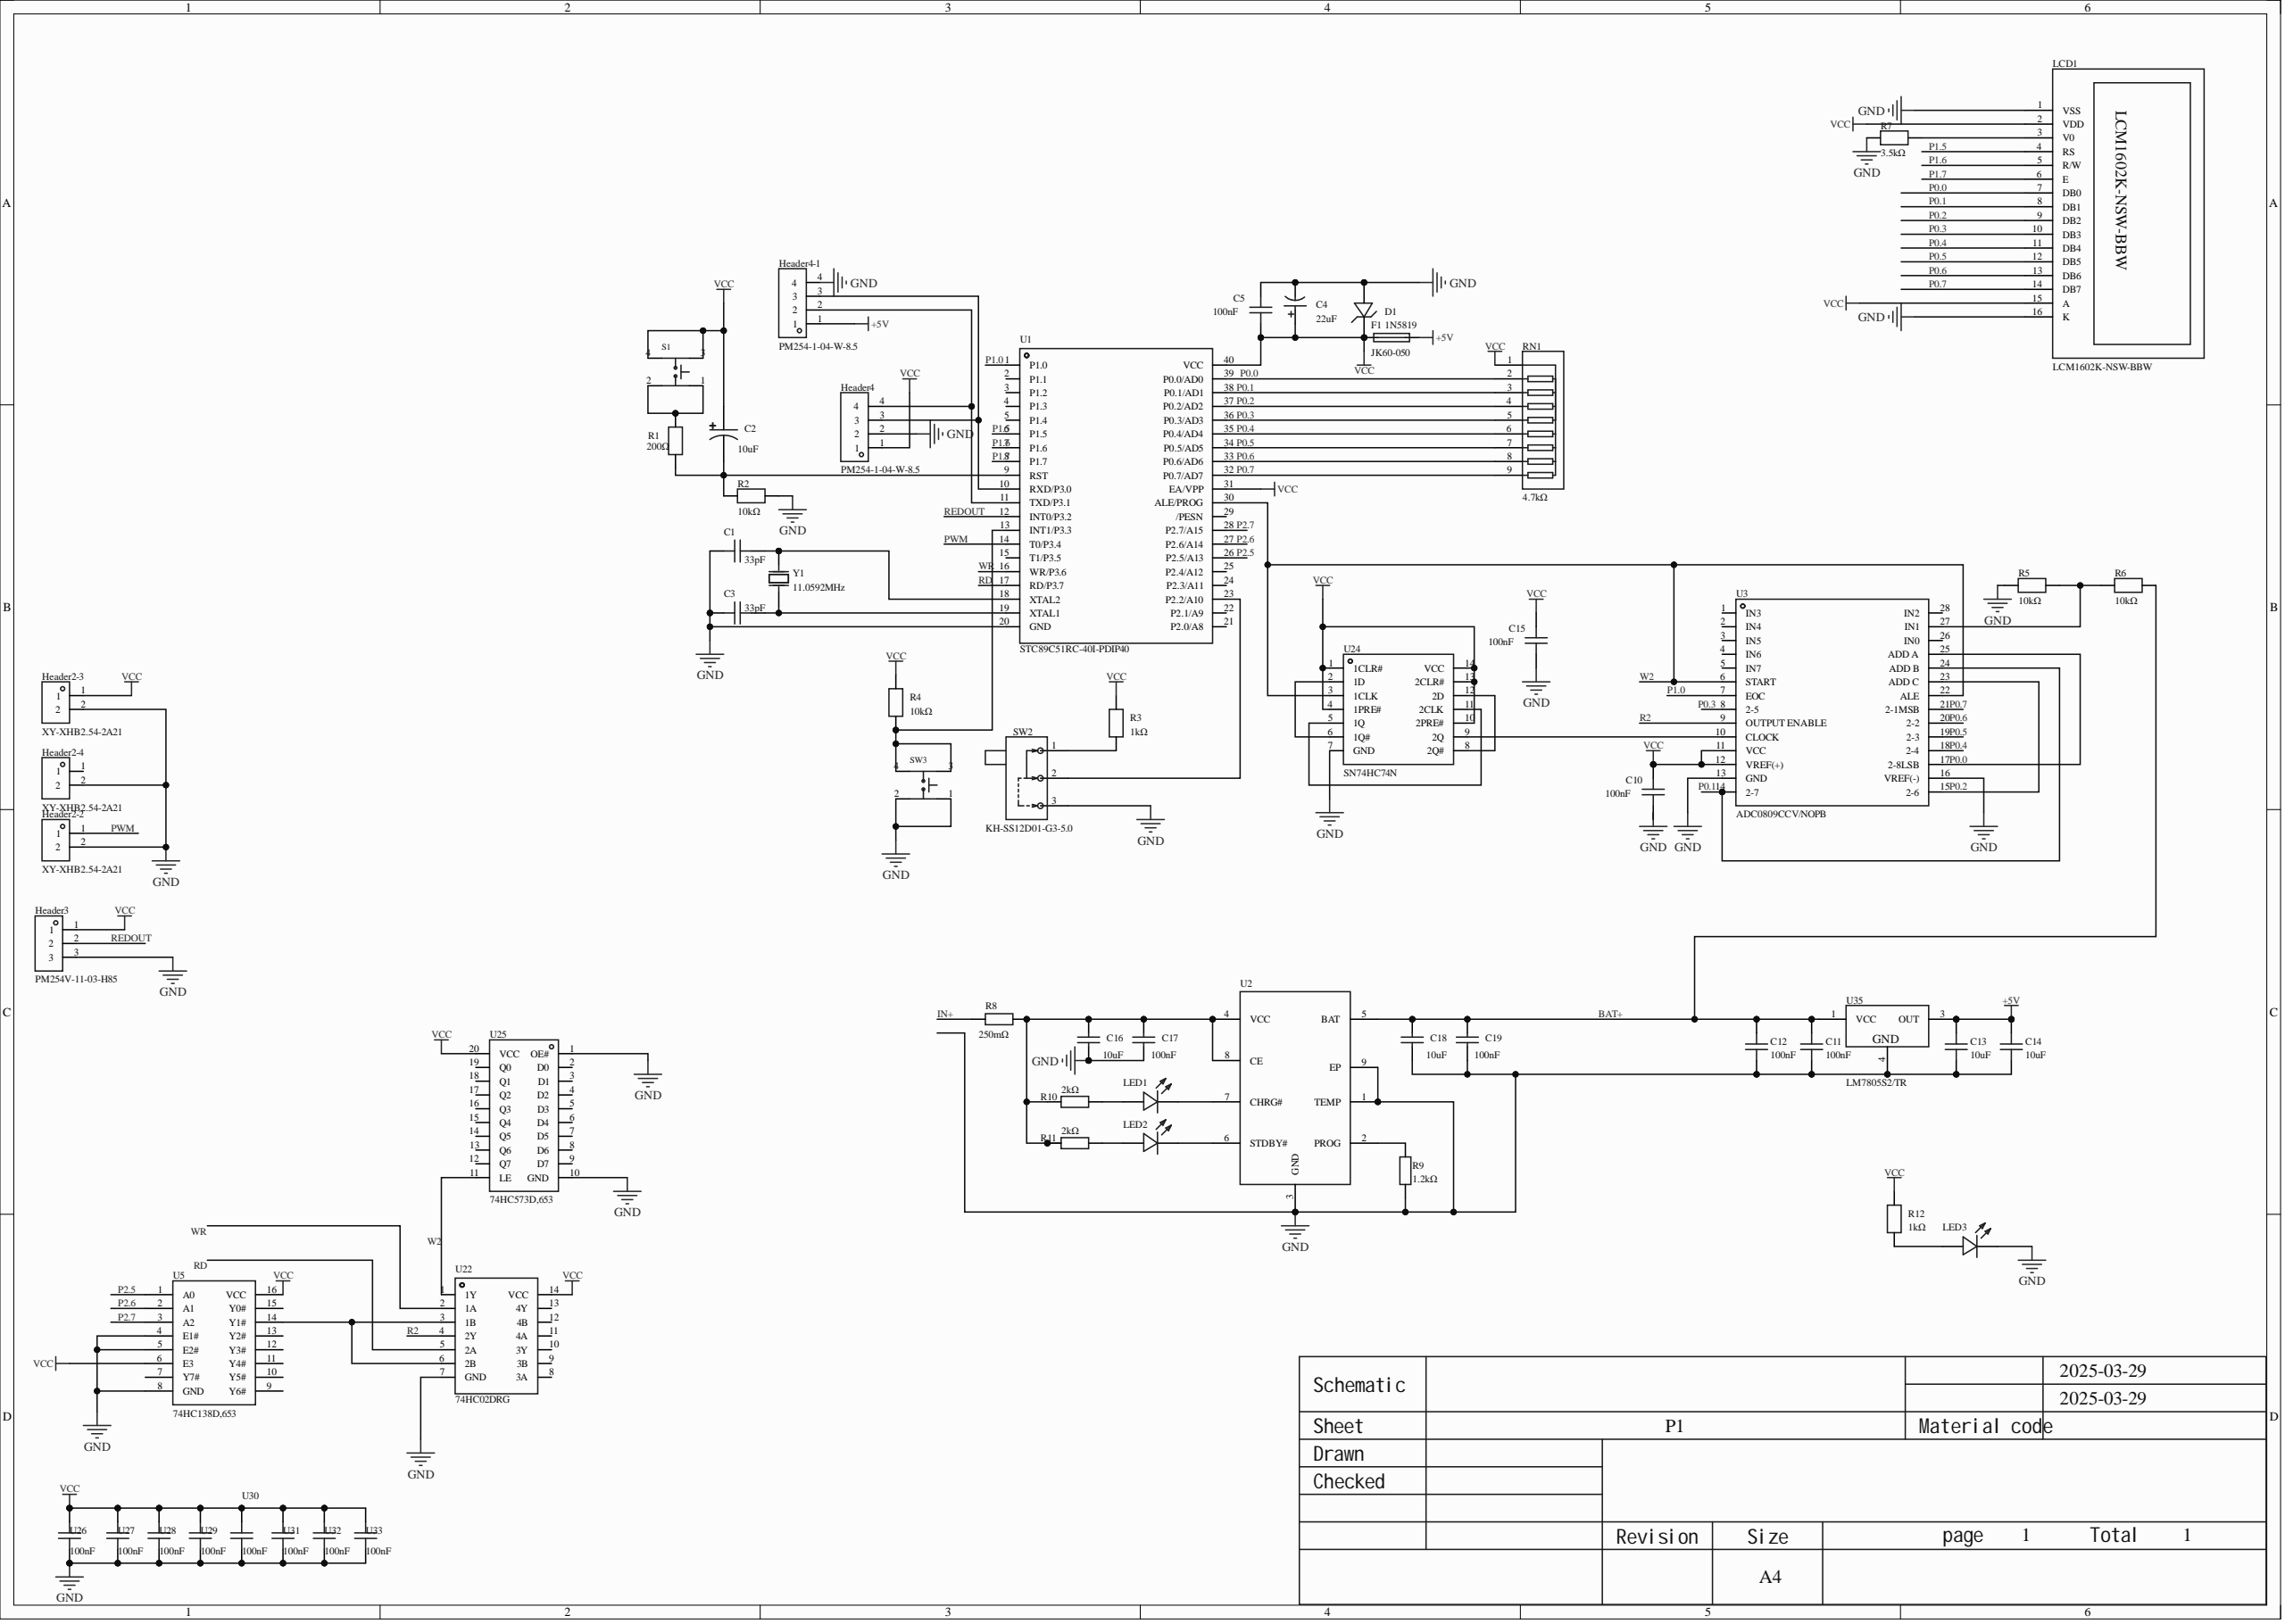Circuit board | Altium Designer | 60 parts | 48 nets
Bill of materials:
Comment,Description,Designator,Footprint,LibRef,Quantity
"33pF","Capacitance: 33pF; Tolerance: ±5%; Rated voltage: 50V; Temperature coefficient: C0G;","C1, C3","RAD-0.2","CC4-0805N330J500F3","2"
"10uF","Capacitance: 10uF; Tolerance: ±20%; Rated voltage: 16V; Ripple current: 24mA@120Hz; ESR: -;","C2","RB1-2","KS1C100MB070A00CV0","1"
"22uF","Capacitance: 22uF; Tolerance: ±20%; Rated voltage: 16V; Ripple current: -; ESR: -;","C4","RB1-2","KM226M016D11RR0VH2FP0","1"
"100nF","Capacitance: 100nF; Tolerance: ±10%; Rated voltage: 50V; Temperature coefficient: X7R;, Capacitance: 100nF; Tolerance: ±10%; Rated voltage: 50V; Material (temp. coefficient): X7R;","C5, C10, C11, C12, C15, C17, C19, U26, U27, U28, U29, U30, U31, U32, U33","RAD-0.2","178MU0002, CC0603KRX7R9BB104, CC0805KRX7R9BB104, 178MU0006","15"
"10uF","Capacitance: 10uF; Tolerance: ±20%; Rated voltage: 6.3V; Material (temp. coefficient): X5R;, Capacitance: 10uF; Tolerance: ±10%; Rated voltage: 16V; Material (temp. coefficient): X5R;","C13, C14, C16, C18","RAD-0.2","CL10A106MQ8NNNC, CL21A106KOQNNNE","4"
"1N5819","Forward voltage drop (Vf): 900mV@3A; DC reverse voltage (Vr): 40V; Average rectified current (Io): 1A;","D1","DIODE-3","1N5819_C402218","1"
"JK60-050","Max voltage: 60V; Max current: 40A; Hold current: 500mA; Trip current: 1A;","F1","FUSE-2","JK60-050","1"
"XY-XHB2.54-2A21","Pin structure: 1x2P; Pitch: 2.54mm; Mounting: right-angle; Total pins: 2P; Rows: 1; Pins per row: 2; Row spacing: 2.54mm; Rated current: 2A; Operating temperature: -25℃~+85℃;","Header2-2, Header2-3, Header2-4","CON2-5","XY-XHB2.54-2A21","3"
"PM254V-11-03-H85","Hole structure: 1x3P; Pitch: 2.54mm; Row spacing: -; Mounting: through-hole; Rows: single row; Total holes: 3P; Plastic height: -; Contact material: brass; Contact plating: -;","Header3","CON3","PM254V-11-03-H85","1"
"PM254-1-04-W-8.5","插孔结构:1x4P;间距:2.54mm;行距:-;圆孔/方孔:方孔;安装类型:弯插;排数:单排;总孔位数:4P;额定电流:3A;额定电压:-;插孔方向:侧面;塑高:8.5mm;触头材质:铜合金;工作温度范围:-40℃~+105℃;焊接温度(最大值):260℃@5S;","Header4, Header4-1","CON4","PM254-1-04-W-8.5","2"
"LCM1602K-NSW-BBW","Main controller chip: KS0066U; Size (inch): -;","LCD1","LCD1602","LCM1602K-NSW-BBW","1"
"204-10SYGD/S530-E3","Lamp head type: 3mm round lamp head; Emitted color: yellow-green;","LED1, LED3","LED1","204-10SYGD/S530-E3","2"
"333-2SYGD/S530-E2-L","灯头类型:5mm圆形灯头;发光颜色:黄绿色;功率:60mW;正向电流:20mA;主波长:573nm;二极管配置:-;透镜颜色:雾状绿透镜;色温:-;发光角度:45°;载带方式:-;工作温度:-40℃~+85℃;","LED2","LED1","333-2SYGD/S530-E2-L","1"
"200Ω","Resistor type: Metal film resistor; Resistance: 200Ω; Tolerance: ±1%; Power: 2W; Temperature coefficient: ±200ppm/?;","R1","AXIAL-0.3","MF2WS-200Ω±1%T","1"
"10kΩ","Resistor type: Metal film resistor; Resistance: 10kΩ; Tolerance: ±1%; Power: 250mW; Temperature coefficient: ±50ppm/?;","R2, R4, R5, R6","AXIAL-0.3","RN1/4W10KFT/BA1","4"
"1kΩ","Resistor type: Metal film resistor; Resistance: 1kΩ; Tolerance: ±1%; Power: 250mW; Temperature coefficient: ±200ppm/?;","R3, R12","AXIAL-0.3","MF1/4W-1KΩ±1%T52","2"
"3.5kΩ","Resistor type: Metal film resistor; Resistance: 3.5kΩ; Tolerance: ±1%; Power: 125mW; Temperature coefficient: ±100ppm/?;","R7","AXIAL-0.3","MF1/8W-3K5±1%-ST52","1"
"250mΩ","","R8","AXIAL-0.3","25121WF250LT4E","1"
"1.2kΩ","","R9","AXIAL-0.3","0805W8F1201T5E","1"
"2kΩ","","R10, R11","AXIAL-0.3","0805W8F2001T5E","2"
"4.7kΩ","Resistor count: 8; Resistance: 4.7kΩ; Tolerance: ±5%; Power per element: 125mW; Temperature coefficient: ±100ppm/?;","RN1","RP","A09-472JP","1"
"","Circuit: SPST; Button shape: round button; Mounting: through-hole; Switch length: 6mm; Switch width: 6mm; Switch height: 5mm; Contact current: 50mA; Rated voltage (DC): 12V; Illuminated: -; Mechanical life: -;","S1, SW3","RST","SKHHAKA010","2"
"KH-SS12D01-G3-5.0","","SW2","RT","KH-SS12D01-G3-5.0","1"
"STC89C51RC-40I-PDIP40","","U1","DIP-40","STC89C51RC-40I-PDIP40","1"
"TP4056-42-ESOP8","Battery type: -; Battery cells: -; Max charge current: -; Full-charge voltage: -; Max supply voltage: -;","U2","ESOP-8_L4.9-W3.9-P1.27-LS6.0-BL-EP","TP4056-42-ESOP8","1"
"ADC0809CCV/NOPB","Interface: parallel; Supply voltage: 4.5V~6.5V; Sampling rate: 10kHz; Resolution: 8-bit;","U3","DIP-28","ADC0809CCV/NOPB","1"
"74HC138D,653","Supply voltage: 2V~6V; Channels: 3~8; Sink current (IOL): 5.2mA; Source current (IOH): 5.2mA;","U5","DIP-16","74HC138D,653","1"
"74HC02DRG","Logic type: NOR gate; Channels: 4;","U22","DIP-14","74HC02DRG","1"
"SN74HC74N","Type: D-type; Supply voltage: 2V~6V; Clock frequency: 60MHz; Elements: 2; Bits per element: 1; Max propagation delay: 30ns@6V,50pF; Quiescent current (Iq): 4uA;","U24","DIP-14","SN74HC74N","1"
"74HC573D,653","Logic type: D-type latch; Supply voltage: 2V~6V; Propagation delay: 14ns;","U25","DIP-20","74HC573D,653","1"
"LM7805S2/TR","","U35","TO-263-2_L10.0-W9.1-P5.08-LS15.2-BL","LM7805S2/TR","1"
"11.059MHz","Crystal type: through-hole crystal; Frequency: 11.059MHz; Frequency tolerance (room temp): ±20ppm; Load capacitance: 20pF; Frequency stability (full temp): ±30ppm;","Y1","XTAL-2","X49SD110592MSD2SC","1"
Netlist (Protel format):
[
C1
RAD-0.2
33pF



]
[
C2
RB1-2
10uF



]
[
C3
RAD-0.2
33pF



]
[
C4
RB1-2
22uF



]
[
C5
RAD-0.2
100nF



]
[
C10
RAD-0.2
100nF



]
[
C11
RAD-0.2
100nF



]
[
C12
RAD-0.2
100nF



]
[
C13
RAD-0.2
10uF



]
[
C14
RAD-0.2
10uF



]
[
C15
RAD-0.2
100nF



]
[
C16
RAD-0.2
10uF



]
[
C17
RAD-0.2
100nF



]
[
C18
RAD-0.2
10uF



]
[
C19
RAD-0.2
100nF



]
[
D1
DIODE-3
1N5819



]
[
F1
FUSE-2
JK60-050



]
[
Header2-2
CON2-5
XY-XHB2.54-2A21



]
[
Header2-3
CON2-5
XY-XHB2.54-2A21



]
[
Header2-4
CON2-5
XY-XHB2.54-2A21



]
[
Header3
CON3
PM254V-11-03-H85



]
[
Header4
CON4
PM254-1-04-W-8.5



]
[
Header4-1
CON4
PM254-1-04-W-8.5



]
[
LCD1
LCD1602
LCM1602K-NSW-BBW



]
[
LED1
LED1
204-10SYGD/S530-E3



]
[
LED2
LED1
333-2SYGD/S530-E2-L



]
[
LED3
LED1
204-10SYGD/S530-E3



]
[
R1
AXIAL-0.3
200Ω



]
[
R2
AXIAL-0.3
10kΩ



]
[
R3
AXIAL-0.3
1kΩ



]
[
R4
AXIAL-0.3
10kΩ



]
[
R5
AXIAL-0.3
10kΩ



]
[
R6
AXIAL-0.3
10kΩ



]
[
R7
AXIAL-0.3
3.5kΩ



]
[
R8
AXIAL-0.3
250mΩ



]
[
R9
AXIAL-0.3
1.2kΩ



]
[
R10
AXIAL-0.3
2kΩ



]
[
R11
AXIAL-0.3
2kΩ



]
[
R12
AXIAL-0.3
1kΩ



]
[
RN1
RP
4.7kΩ



]
[
S1
RST




]
[
SW2
RT
KH-SS12D01-G3-5.0



]
[
SW3
RST




]
[
U1
DIP-40
STC89C51RC-40I-PDIP40



]
[
U2
ESOP-8_L4.9-W3.9-P1.27-LS6.0-BL-EP
TP4056-42-ESOP8



]
[
U3
DIP-28
ADC0809CCV/NOPB



]
[
U5
DIP-16
74HC138D,653



]
[
U22
DIP-14
74HC02DRG



]
[
U24
DIP-14
SN74HC74N



]
[
U25
DIP-20
74HC573D,653



]
[
U26
RAD-0.2
100nF



]
[
U27
RAD-0.2
100nF



]
[
U28
RAD-0.2
100nF



]
[
U29
RAD-0.2
100nF



]
[
U30
RAD-0.2
100nF



]
[
U31
RAD-0.2
100nF



]
[
U32
RAD-0.2
100nF



]
[
U33
RAD-0.2
100nF



]
[
U35
TO-263-2_L10.0-W9.1-P5.08-LS15.2-BL
LM7805S2/TR



]
[
Y1
XTAL-2
11.0592MHz



]
(
WR
U1-16
U22-2
)
(
W2
U1-30
U3-6
U3-22
U22-1
U24-3
U25-11
)
(
VCC
C2-1
C4-1
C5-1
C10-2
C15-2
D1-1
F1-1
Header2-3-1
Header3-1
Header4-1
LCD1-2
LCD1-15
R3-2
R4-2
R12-2
RN1-1
S1-3
S1-4
U1-31
U1-40
U3-11
U3-12
U5-6
U5-16
U22-14
U24-1
U24-4
U24-10
U24-13
U24-14
U25-20
U26-2
U27-2
U28-2
U29-2
U30-2
U31-2
U32-2
U33-2
)
(
REDOUT
Header3-2
U1-12
)
(
RD
U1-17
U22-5
)
(
R2
U3-9
U22-4
)
(
PWM
Header2-2-1
U1-14
)
(
P2.7
U1-28
U5-3
)
(
P2.6
U1-27
U5-2
)
(
P2.5
U1-26
U5-1
)
(
P1.7
LCD1-6
U1-8
)
(
P1.6
LCD1-5
U1-7
)
(
P1.5
LCD1-4
U1-6
)
(
P1.0
U1-1
U3-7
)
(
P0.7
LCD1-14
RN1-9
U1-32
U3-21
)
(
P0.6
LCD1-13
RN1-8
U1-33
U3-20
)
(
P0.5
LCD1-12
RN1-7
U1-34
U3-19
)
(
P0.4
LCD1-11
RN1-6
U1-35
U3-18
)
(
P0.3
LCD1-10
RN1-5
U1-36
U3-8
)
(
P0.2
LCD1-9
RN1-4
U1-37
U3-15
U3-23
)
(
P0.1
LCD1-8
RN1-3
U1-38
U3-14
U3-24
)
(
P0.0
LCD1-7
RN1-2
U1-39
U3-17
U3-25
)
(
NetU24_8
U24-8
U24-12
)
(
NetU24_5
U24-5
U24-11
)
(
NetU24_2
U24-2
U24-6
)
(
NetU5_14
U5-14
U22-3
U22-6
)
(
NetU3_10
U3-10
U24-9
)
(
NetSW2_2
SW2-2
U1-23
)
(
NetR9_2
R9-2
U2-2
)
(
NetR5_2
R5-2
R6-1
U3-27
)
(
NetR4_1
R4-1
SW3-3
SW3-4
U1-13
)
(
NetR3_1
R3-1
SW2-1
)
(
NetR1_1
R1-1
S1-1
S1-2
)
(
NetLED3_1
LED3-1
R12-1
)
(
NetLED2_2
LED2-2
R11-2
)
(
NetLED2_1
LED2-1
U2-6
)
(
NetLED1_2
LED1-2
U2-7
)
(
NetLED1_1
LED1-1
R10-2
)
(
NetLCD1_3
LCD1-3
R7-2
)
(
NetHeader4-1_3
Header4-3
Header4-1-3
U1-10
)
(
NetHeader4-1_2
Header4-4
Header4-1-2
U1-11
)
(
NetC16_2
C16-2
C17-2
R8-2
R10-1
R11-1
U2-4
U2-8
)
(
NetC3_1
C3-1
U1-19
Y1-2
)
(
NetC2_2
C2-2
R1-2
R2-1
U1-9
)
(
NetC1_1
C1-1
U1-18
Y1-1
)
(
GND
C1-2
C3-2
C4-2
C5-2
C10-1
C11-1
C12-1
C13-1
C14-1
C15-1
C16-1
C17-1
C18-1
C19-1
D1-2
Header2-2-2
Header2-3-2
Header2-4-2
Header3-3
Header4-2
Header4-1-4
LCD1-1
LCD1-16
LED3-2
R2-2
R5-1
R7-1
R9-1
SW2-3
SW3-1
SW3-2
U1-20
U2-1
U2-3
U2-9
U3-13
U3-16
U5-4
U5-5
U5-8
U22-7
U24-7
U25-1
U25-10
U26-1
U27-1
U28-1
U29-1
U30-1
U31-1
U32-1
U33-1
U35-4
)
(
BAT+
C11-2
C12-2
C18-2
C19-2
R6-2
U2-5
U35-1
)
(
+5V
C13-2
C14-2
F1-2
Header4-1-1
U35-3
)